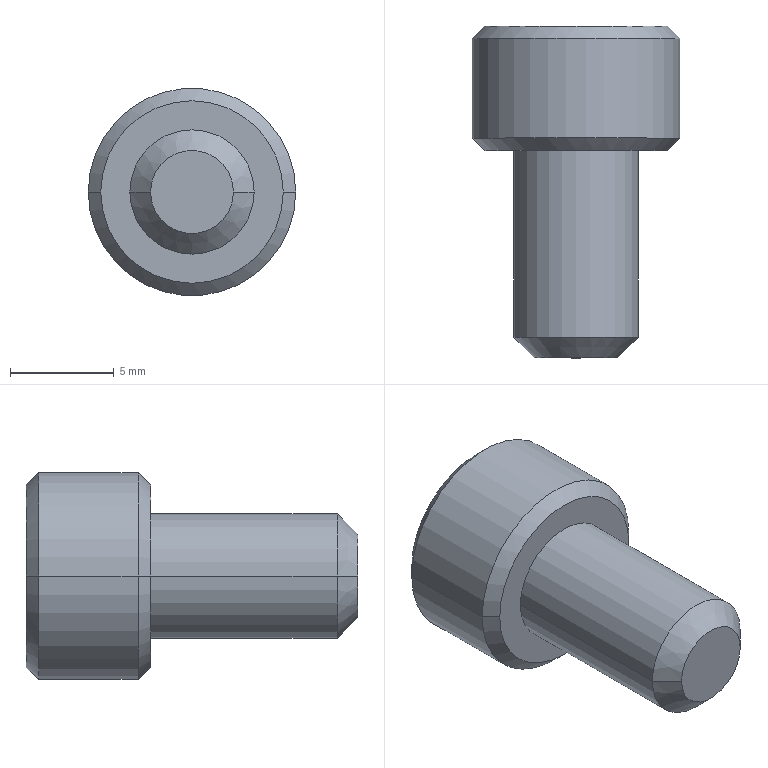Part | STEP file | BB62-M6-10L-3 | 1 solid | 27 faces | box 10 x 16 x 10 mm | volume 656.85 mm3 | plane 15 | cone 8 | cylinder 4 | commonest cylinder face diameters 6 x2 10 x2
STEP:
#1=CARTESIAN_POINT('',(0.,1.349,0.));
#2=VERTEX_POINT('',#1);
#3=CARTESIAN_POINT('',(2.86,3.,0.));
#4=VERTEX_POINT('',#3);
#5=CARTESIAN_POINT('',(0.,1.349,0.));
#6=DIRECTION('',(0.866,0.5,0.));
#7=VECTOR('',#6,1000.);
#8=LINE('',#5,#7);
#9=EDGE_CURVE('',#2,#4,#8,.T.);
#10=ORIENTED_EDGE('',*,*,#9,.F.);
#11=CARTESIAN_POINT('',(-2.86,3.,0.));
#12=VERTEX_POINT('',#11);
#13=CARTESIAN_POINT('',(0.,1.349,0.));
#14=DIRECTION('',(-0.866,0.5,0.));
#15=VECTOR('',#14,1000.);
#16=LINE('',#13,#15);
#17=EDGE_CURVE('',#2,#12,#16,.T.);
#18=ORIENTED_EDGE('',*,*,#17,.T.);
#19=CARTESIAN_POINT('',(-2.477,3.,1.43));
#20=VERTEX_POINT('',#19);
#21=CARTESIAN_POINT('',(0.,3.,0.));
#22=DIRECTION('',(0.,-1.,0.));
#23=DIRECTION('',(-1.,0.,0.));
#24=AXIS2_PLACEMENT_3D('',#21,#22,#23);
#25=CIRCLE('',#24,2.86);
#26=EDGE_CURVE('',#20,#12,#25,.T.);
#27=ORIENTED_EDGE('',*,*,#26,.F.);
#28=CARTESIAN_POINT('',(0.,3.,2.86));
#29=VERTEX_POINT('',#28);
#30=CARTESIAN_POINT('',(0.,3.,0.));
#31=DIRECTION('',(0.,-1.,0.));
#32=DIRECTION('',(-1.,0.,0.));
#33=AXIS2_PLACEMENT_3D('',#30,#31,#32);
#34=CIRCLE('',#33,2.86);
#35=EDGE_CURVE('',#29,#20,#34,.T.);
#36=ORIENTED_EDGE('',*,*,#35,.F.);
#37=CARTESIAN_POINT('',(2.477,3.,1.43));
#38=VERTEX_POINT('',#37);
#39=CARTESIAN_POINT('',(0.,3.,0.));
#40=DIRECTION('',(0.,-1.,0.));
#41=DIRECTION('',(-1.,0.,0.));
#42=AXIS2_PLACEMENT_3D('',#39,#40,#41);
#43=CIRCLE('',#42,2.86);
#44=EDGE_CURVE('',#38,#29,#43,.T.);
#45=ORIENTED_EDGE('',*,*,#44,.F.);
#46=CARTESIAN_POINT('',(0.,3.,0.));
#47=DIRECTION('',(0.,-1.,0.));
#48=DIRECTION('',(-1.,0.,0.));
#49=AXIS2_PLACEMENT_3D('',#46,#47,#48);
#50=CIRCLE('',#49,2.86);
#51=EDGE_CURVE('',#4,#38,#50,.T.);
#52=ORIENTED_EDGE('',*,*,#51,.F.);
#53=EDGE_LOOP('',(#10,#18,#27,#36,#45,#52));
#54=FACE_OUTER_BOUND('',#53,.T.);
#55=CARTESIAN_POINT('',(0.,1001.349,0.));
#56=DIRECTION('',(0.,1.,0.));
#57=DIRECTION('',(1.,0.,0.));
#58=AXIS2_PLACEMENT_3D('',#55,#56,#57);
#59=CONICAL_SURFACE('',#58,1732.051,1.047);
#60=ADVANCED_FACE('',(#54),#59,.F.);
#61=CARTESIAN_POINT('',(2.,-10.,0.));
#62=VERTEX_POINT('',#61);
#63=CARTESIAN_POINT('',(-2.,-10.,0.));
#64=VERTEX_POINT('',#63);
#65=CARTESIAN_POINT('',(0.,-10.,0.));
#66=DIRECTION('',(0.,1.,0.));
#67=DIRECTION('',(1.,0.,0.));
#68=AXIS2_PLACEMENT_3D('',#65,#66,#67);
#69=CIRCLE('',#68,2.);
#70=EDGE_CURVE('',#62,#64,#69,.T.);
#71=ORIENTED_EDGE('',*,*,#70,.T.);
#72=CARTESIAN_POINT('',(-3.,-9.,0.));
#73=VERTEX_POINT('',#72);
#74=CARTESIAN_POINT('',(-2.,-10.,0.));
#75=DIRECTION('',(-0.7071,0.7071,0.));
#76=VECTOR('',#75,1000.);
#77=LINE('',#74,#76);
#78=EDGE_CURVE('',#64,#73,#77,.T.);
#79=ORIENTED_EDGE('',*,*,#78,.T.);
#80=CARTESIAN_POINT('',(3.,-9.,0.));
#81=VERTEX_POINT('',#80);
#82=CARTESIAN_POINT('',(0.,-9.,0.));
#83=DIRECTION('',(0.,-1.,0.));
#84=DIRECTION('',(-1.,0.,0.));
#85=AXIS2_PLACEMENT_3D('',#82,#83,#84);
#86=CIRCLE('',#85,3.);
#87=EDGE_CURVE('',#73,#81,#86,.T.);
#88=ORIENTED_EDGE('',*,*,#87,.T.);
#89=CARTESIAN_POINT('',(2.,-10.,0.));
#90=DIRECTION('',(0.7071,0.7071,0.));
#91=VECTOR('',#90,1000.);
#92=LINE('',#89,#91);
#93=EDGE_CURVE('',#62,#81,#92,.T.);
#94=ORIENTED_EDGE('',*,*,#93,.F.);
#95=EDGE_LOOP('',(#71,#79,#88,#94));
#96=FACE_OUTER_BOUND('',#95,.T.);
#97=CARTESIAN_POINT('',(0.,-10.,0.));
#98=DIRECTION('',(0.,1.,0.));
#99=DIRECTION('',(1.,0.,0.));
#100=AXIS2_PLACEMENT_3D('',#97,#98,#99);
#101=CONICAL_SURFACE('',#100,2.,0.7854);
#102=ADVANCED_FACE('',(#96),#101,.T.);
#103=ORIENTED_EDGE('',*,*,#87,.F.);
#104=CARTESIAN_POINT('',(-3.,0.,0.));
#105=VERTEX_POINT('',#104);
#106=CARTESIAN_POINT('',(-3.,-9.,0.));
#107=DIRECTION('',(0.,1.,0.));
#108=VECTOR('',#107,1000.);
#109=LINE('',#106,#108);
#110=EDGE_CURVE('',#73,#105,#109,.T.);
#111=ORIENTED_EDGE('',*,*,#110,.T.);
#112=CARTESIAN_POINT('',(3.,0.,0.));
#113=VERTEX_POINT('',#112);
#114=CARTESIAN_POINT('',(0.,0.,0.));
#115=DIRECTION('',(0.,-1.,0.));
#116=DIRECTION('',(-1.,0.,0.));
#117=AXIS2_PLACEMENT_3D('',#114,#115,#116);
#118=CIRCLE('',#117,3.);
#119=EDGE_CURVE('',#105,#113,#118,.T.);
#120=ORIENTED_EDGE('',*,*,#119,.T.);
#121=CARTESIAN_POINT('',(3.,-9.,0.));
#122=DIRECTION('',(0.,1.,0.));
#123=VECTOR('',#122,1000.);
#124=LINE('',#121,#123);
#125=EDGE_CURVE('',#81,#113,#124,.T.);
#126=ORIENTED_EDGE('',*,*,#125,.F.);
#127=EDGE_LOOP('',(#103,#111,#120,#126));
#128=FACE_OUTER_BOUND('',#127,.T.);
#129=CARTESIAN_POINT('',(0.,-9.,0.));
#130=DIRECTION('',(0.,1.,0.));
#131=DIRECTION('',(1.,0.,0.));
#132=AXIS2_PLACEMENT_3D('',#129,#130,#131);
#133=CYLINDRICAL_SURFACE('',#132,3.);
#134=ADVANCED_FACE('',(#128),#133,.T.);
#135=CARTESIAN_POINT('',(-4.4,6.,0.));
#136=VERTEX_POINT('',#135);
#137=CARTESIAN_POINT('',(4.4,6.,0.));
#138=VERTEX_POINT('',#137);
#139=CARTESIAN_POINT('',(0.,6.,0.));
#140=DIRECTION('',(0.,-1.,0.));
#141=DIRECTION('',(-1.,0.,0.));
#142=AXIS2_PLACEMENT_3D('',#139,#140,#141);
#143=CIRCLE('',#142,4.4);
#144=EDGE_CURVE('',#136,#138,#143,.T.);
#145=ORIENTED_EDGE('',*,*,#144,.T.);
#146=CARTESIAN_POINT('',(5.,5.4,0.));
#147=VERTEX_POINT('',#146);
#148=CARTESIAN_POINT('',(5.,5.4,0.));
#149=DIRECTION('',(0.7071,-0.7071,0.));
#150=VECTOR('',#149,1000.);
#151=LINE('',#148,#150);
#152=EDGE_CURVE('',#138,#147,#151,.T.);
#153=ORIENTED_EDGE('',*,*,#152,.T.);
#154=CARTESIAN_POINT('',(-5.,5.4,0.));
#155=VERTEX_POINT('',#154);
#156=CARTESIAN_POINT('',(0.,5.4,0.));
#157=DIRECTION('',(0.,-1.,0.));
#158=DIRECTION('',(-1.,0.,0.));
#159=AXIS2_PLACEMENT_3D('',#156,#157,#158);
#160=CIRCLE('',#159,5.);
#161=EDGE_CURVE('',#155,#147,#160,.T.);
#162=ORIENTED_EDGE('',*,*,#161,.F.);
#163=CARTESIAN_POINT('',(-5.,5.4,0.));
#164=DIRECTION('',(-0.7071,-0.7071,0.));
#165=VECTOR('',#164,1000.);
#166=LINE('',#163,#165);
#167=EDGE_CURVE('',#136,#155,#166,.T.);
#168=ORIENTED_EDGE('',*,*,#167,.F.);
#169=EDGE_LOOP('',(#145,#153,#162,#168));
#170=FACE_OUTER_BOUND('',#169,.T.);
#171=CARTESIAN_POINT('',(0.,5.4,0.));
#172=DIRECTION('',(0.,-1.,0.));
#173=DIRECTION('',(-1.,0.,0.));
#174=AXIS2_PLACEMENT_3D('',#171,#172,#173);
#175=CONICAL_SURFACE('',#174,5.,0.7854);
#176=ADVANCED_FACE('',(#170),#175,.T.);
#177=ORIENTED_EDGE('',*,*,#161,.T.);
#178=CARTESIAN_POINT('',(5.,0.6,0.));
#179=VERTEX_POINT('',#178);
#180=CARTESIAN_POINT('',(5.,1.62,0.));
#181=DIRECTION('',(0.,-1.,0.));
#182=VECTOR('',#181,1000.);
#183=LINE('',#180,#182);
#184=EDGE_CURVE('',#147,#179,#183,.T.);
#185=ORIENTED_EDGE('',*,*,#184,.T.);
#186=CARTESIAN_POINT('',(-5.,0.6,0.));
#187=VERTEX_POINT('',#186);
#188=CARTESIAN_POINT('',(0.,0.6,0.));
#189=DIRECTION('',(0.,-1.,0.));
#190=DIRECTION('',(-1.,0.,0.));
#191=AXIS2_PLACEMENT_3D('',#188,#189,#190);
#192=CIRCLE('',#191,5.);
#193=EDGE_CURVE('',#187,#179,#192,.T.);
#194=ORIENTED_EDGE('',*,*,#193,.F.);
#195=CARTESIAN_POINT('',(-5.,1.62,0.));
#196=DIRECTION('',(0.,-1.,0.));
#197=VECTOR('',#196,1000.);
#198=LINE('',#195,#197);
#199=EDGE_CURVE('',#155,#187,#198,.T.);
#200=ORIENTED_EDGE('',*,*,#199,.F.);
#201=EDGE_LOOP('',(#177,#185,#194,#200));
#202=FACE_OUTER_BOUND('',#201,.T.);
#203=CARTESIAN_POINT('',(0.,1.62,0.));
#204=DIRECTION('',(0.,-1.,0.));
#205=DIRECTION('',(-1.,0.,0.));
#206=AXIS2_PLACEMENT_3D('',#203,#204,#205);
#207=CYLINDRICAL_SURFACE('',#206,5.);
#208=ADVANCED_FACE('',(#202),#207,.T.);
#209=CARTESIAN_POINT('',(-4.4,0.,0.));
#210=VERTEX_POINT('',#209);
#211=CARTESIAN_POINT('',(4.4,0.,0.));
#212=VERTEX_POINT('',#211);
#213=CARTESIAN_POINT('',(0.,0.,0.));
#214=DIRECTION('',(0.,-1.,0.));
#215=DIRECTION('',(-1.,0.,0.));
#216=AXIS2_PLACEMENT_3D('',#213,#214,#215);
#217=CIRCLE('',#216,4.4);
#218=EDGE_CURVE('',#210,#212,#217,.T.);
#219=ORIENTED_EDGE('',*,*,#218,.F.);
#220=CARTESIAN_POINT('',(-4.4,0.,0.));
#221=DIRECTION('',(-0.7071,0.7071,0.));
#222=VECTOR('',#221,1000.);
#223=LINE('',#220,#222);
#224=EDGE_CURVE('',#210,#187,#223,.T.);
#225=ORIENTED_EDGE('',*,*,#224,.T.);
#226=ORIENTED_EDGE('',*,*,#193,.T.);
#227=CARTESIAN_POINT('',(4.4,0.,0.));
#228=DIRECTION('',(0.7071,0.7071,0.));
#229=VECTOR('',#228,1000.);
#230=LINE('',#227,#229);
#231=EDGE_CURVE('',#212,#179,#230,.T.);
#232=ORIENTED_EDGE('',*,*,#231,.F.);
#233=EDGE_LOOP('',(#219,#225,#226,#232));
#234=FACE_OUTER_BOUND('',#233,.T.);
#235=CARTESIAN_POINT('',(0.,0.,0.));
#236=DIRECTION('',(0.,1.,0.));
#237=DIRECTION('',(1.,0.,0.));
#238=AXIS2_PLACEMENT_3D('',#235,#236,#237);
#239=CONICAL_SURFACE('',#238,4.4,0.7854);
#240=ADVANCED_FACE('',(#234),#239,.T.);
#241=ORIENTED_EDGE('',*,*,#144,.F.);
#242=CARTESIAN_POINT('',(0.,6.,0.));
#243=DIRECTION('',(0.,-1.,0.));
#244=DIRECTION('',(-1.,0.,0.));
#245=AXIS2_PLACEMENT_3D('',#242,#243,#244);
#246=CIRCLE('',#245,4.4);
#247=EDGE_CURVE('',#138,#136,#246,.T.);
#248=ORIENTED_EDGE('',*,*,#247,.F.);
#249=EDGE_LOOP('',(#241,#248));
#250=FACE_OUTER_BOUND('',#249,.T.);
#251=CARTESIAN_POINT('',(0.,6.,-2.86));
#252=VERTEX_POINT('',#251);
#253=CARTESIAN_POINT('',(-2.477,6.,-1.43));
#254=VERTEX_POINT('',#253);
#255=CARTESIAN_POINT('',(0.,6.,-2.86));
#256=DIRECTION('',(-0.866,0.,0.5));
#257=VECTOR('',#256,1000.);
#258=LINE('',#255,#257);
#259=EDGE_CURVE('',#252,#254,#258,.T.);
#260=ORIENTED_EDGE('',*,*,#259,.F.);
#261=CARTESIAN_POINT('',(2.477,6.,-1.43));
#262=VERTEX_POINT('',#261);
#263=CARTESIAN_POINT('',(2.477,6.,-1.43));
#264=DIRECTION('',(-0.866,0.,-0.5));
#265=VECTOR('',#264,1000.);
#266=LINE('',#263,#265);
#267=EDGE_CURVE('',#262,#252,#266,.T.);
#268=ORIENTED_EDGE('',*,*,#267,.F.);
#269=CARTESIAN_POINT('',(2.477,6.,1.43));
#270=VERTEX_POINT('',#269);
#271=CARTESIAN_POINT('',(2.477,6.,1.43));
#272=DIRECTION('',(0.,0.,-1.));
#273=VECTOR('',#272,1000.);
#274=LINE('',#271,#273);
#275=EDGE_CURVE('',#270,#262,#274,.T.);
#276=ORIENTED_EDGE('',*,*,#275,.F.);
#277=CARTESIAN_POINT('',(0.,6.,2.86));
#278=VERTEX_POINT('',#277);
#279=CARTESIAN_POINT('',(0.,6.,2.86));
#280=DIRECTION('',(0.866,0.,-0.5));
#281=VECTOR('',#280,1000.);
#282=LINE('',#279,#281);
#283=EDGE_CURVE('',#278,#270,#282,.T.);
#284=ORIENTED_EDGE('',*,*,#283,.F.);
#285=CARTESIAN_POINT('',(-2.477,6.,1.43));
#286=VERTEX_POINT('',#285);
#287=CARTESIAN_POINT('',(-2.477,6.,1.43));
#288=DIRECTION('',(0.866,0.,0.5));
#289=VECTOR('',#288,1000.);
#290=LINE('',#287,#289);
#291=EDGE_CURVE('',#286,#278,#290,.T.);
#292=ORIENTED_EDGE('',*,*,#291,.F.);
#293=CARTESIAN_POINT('',(-2.477,6.,-1.43));
#294=DIRECTION('',(0.,0.,1.));
#295=VECTOR('',#294,1000.);
#296=LINE('',#293,#295);
#297=EDGE_CURVE('',#254,#286,#296,.T.);
#298=ORIENTED_EDGE('',*,*,#297,.F.);
#299=EDGE_LOOP('',(#260,#268,#276,#284,#292,#298));
#300=FACE_BOUND('',#299,.T.);
#301=CARTESIAN_POINT('',(4.4,6.,0.));
#302=DIRECTION('',(0.,1.,0.));
#303=DIRECTION('',(1.,0.,0.));
#304=AXIS2_PLACEMENT_3D('',#301,#302,#303);
#305=PLANE('',#304);
#306=ADVANCED_FACE('',(#250,#300),#305,.T.);
#307=CARTESIAN_POINT('',(0.,0.,0.));
#308=DIRECTION('',(0.,-1.,0.));
#309=DIRECTION('',(-1.,0.,0.));
#310=AXIS2_PLACEMENT_3D('',#307,#308,#309);
#311=CIRCLE('',#310,3.);
#312=EDGE_CURVE('',#113,#105,#311,.T.);
#313=ORIENTED_EDGE('',*,*,#312,.F.);
#314=ORIENTED_EDGE('',*,*,#119,.F.);
#315=EDGE_LOOP('',(#313,#314));
#316=FACE_BOUND('',#315,.T.);
#317=CARTESIAN_POINT('',(0.,0.,0.));
#318=DIRECTION('',(0.,-1.,0.));
#319=DIRECTION('',(-1.,0.,0.));
#320=AXIS2_PLACEMENT_3D('',#317,#318,#319);
#321=CIRCLE('',#320,4.4);
#322=EDGE_CURVE('',#212,#210,#321,.T.);
#323=ORIENTED_EDGE('',*,*,#322,.T.);
#324=ORIENTED_EDGE('',*,*,#218,.T.);
#325=EDGE_LOOP('',(#323,#324));
#326=FACE_OUTER_BOUND('',#325,.T.);
#327=CARTESIAN_POINT('',(0.,0.,0.));
#328=DIRECTION('',(0.,-1.,0.));
#329=DIRECTION('',(-1.,0.,0.));
#330=AXIS2_PLACEMENT_3D('',#327,#328,#329);
#331=PLANE('',#330);
#332=ADVANCED_FACE('',(#316,#326),#331,.T.);
#333=ORIENTED_EDGE('',*,*,#224,.F.);
#334=ORIENTED_EDGE('',*,*,#322,.F.);
#335=ORIENTED_EDGE('',*,*,#231,.T.);
#336=CARTESIAN_POINT('',(0.,0.6,0.));
#337=DIRECTION('',(0.,-1.,0.));
#338=DIRECTION('',(-1.,0.,0.));
#339=AXIS2_PLACEMENT_3D('',#336,#337,#338);
#340=CIRCLE('',#339,5.);
#341=EDGE_CURVE('',#179,#187,#340,.T.);
#342=ORIENTED_EDGE('',*,*,#341,.T.);
#343=EDGE_LOOP('',(#333,#334,#335,#342));
#344=FACE_OUTER_BOUND('',#343,.T.);
#345=CARTESIAN_POINT('',(0.,0.,0.));
#346=DIRECTION('',(0.,1.,0.));
#347=DIRECTION('',(1.,0.,0.));
#348=AXIS2_PLACEMENT_3D('',#345,#346,#347);
#349=CONICAL_SURFACE('',#348,4.4,0.7854);
#350=ADVANCED_FACE('',(#344),#349,.T.);
#351=ORIENTED_EDGE('',*,*,#184,.F.);
#352=CARTESIAN_POINT('',(0.,5.4,0.));
#353=DIRECTION('',(0.,-1.,0.));
#354=DIRECTION('',(-1.,0.,0.));
#355=AXIS2_PLACEMENT_3D('',#352,#353,#354);
#356=CIRCLE('',#355,5.);
#357=EDGE_CURVE('',#147,#155,#356,.T.);
#358=ORIENTED_EDGE('',*,*,#357,.T.);
#359=ORIENTED_EDGE('',*,*,#199,.T.);
#360=ORIENTED_EDGE('',*,*,#341,.F.);
#361=EDGE_LOOP('',(#351,#358,#359,#360));
#362=FACE_OUTER_BOUND('',#361,.T.);
#363=CARTESIAN_POINT('',(0.,1.62,0.));
#364=DIRECTION('',(0.,-1.,0.));
#365=DIRECTION('',(-1.,0.,0.));
#366=AXIS2_PLACEMENT_3D('',#363,#364,#365);
#367=CYLINDRICAL_SURFACE('',#366,5.);
#368=ADVANCED_FACE('',(#362),#367,.T.);
#369=ORIENTED_EDGE('',*,*,#152,.F.);
#370=ORIENTED_EDGE('',*,*,#247,.T.);
#371=ORIENTED_EDGE('',*,*,#167,.T.);
#372=ORIENTED_EDGE('',*,*,#357,.F.);
#373=EDGE_LOOP('',(#369,#370,#371,#372));
#374=FACE_OUTER_BOUND('',#373,.T.);
#375=CARTESIAN_POINT('',(0.,5.4,0.));
#376=DIRECTION('',(0.,-1.,0.));
#377=DIRECTION('',(-1.,0.,0.));
#378=AXIS2_PLACEMENT_3D('',#375,#376,#377);
#379=CONICAL_SURFACE('',#378,5.,0.7854);
#380=ADVANCED_FACE('',(#374),#379,.T.);
#381=ORIENTED_EDGE('',*,*,#110,.F.);
#382=CARTESIAN_POINT('',(0.,-9.,0.));
#383=DIRECTION('',(0.,-1.,0.));
#384=DIRECTION('',(-1.,0.,0.));
#385=AXIS2_PLACEMENT_3D('',#382,#383,#384);
#386=CIRCLE('',#385,3.);
#387=EDGE_CURVE('',#81,#73,#386,.T.);
#388=ORIENTED_EDGE('',*,*,#387,.F.);
#389=ORIENTED_EDGE('',*,*,#125,.T.);
#390=ORIENTED_EDGE('',*,*,#312,.T.);
#391=EDGE_LOOP('',(#381,#388,#389,#390));
#392=FACE_OUTER_BOUND('',#391,.T.);
#393=CARTESIAN_POINT('',(0.,-9.,0.));
#394=DIRECTION('',(0.,1.,0.));
#395=DIRECTION('',(1.,0.,0.));
#396=AXIS2_PLACEMENT_3D('',#393,#394,#395);
#397=CYLINDRICAL_SURFACE('',#396,3.);
#398=ADVANCED_FACE('',(#392),#397,.T.);
#399=ORIENTED_EDGE('',*,*,#70,.F.);
#400=CARTESIAN_POINT('',(0.,-10.,0.));
#401=DIRECTION('',(0.,1.,0.));
#402=DIRECTION('',(1.,0.,0.));
#403=AXIS2_PLACEMENT_3D('',#400,#401,#402);
#404=CIRCLE('',#403,2.);
#405=EDGE_CURVE('',#64,#62,#404,.T.);
#406=ORIENTED_EDGE('',*,*,#405,.F.);
#407=EDGE_LOOP('',(#399,#406));
#408=FACE_OUTER_BOUND('',#407,.T.);
#409=CARTESIAN_POINT('',(0.,-10.,0.));
#410=DIRECTION('',(0.,-1.,0.));
#411=DIRECTION('',(-1.,0.,0.));
#412=AXIS2_PLACEMENT_3D('',#409,#410,#411);
#413=PLANE('',#412);
#414=ADVANCED_FACE('',(#408),#413,.T.);
#415=ORIENTED_EDGE('',*,*,#78,.F.);
#416=ORIENTED_EDGE('',*,*,#405,.T.);
#417=ORIENTED_EDGE('',*,*,#93,.T.);
#418=ORIENTED_EDGE('',*,*,#387,.T.);
#419=EDGE_LOOP('',(#415,#416,#417,#418));
#420=FACE_OUTER_BOUND('',#419,.T.);
#421=CARTESIAN_POINT('',(0.,-10.,0.));
#422=DIRECTION('',(0.,1.,0.));
#423=DIRECTION('',(1.,0.,0.));
#424=AXIS2_PLACEMENT_3D('',#421,#422,#423);
#425=CONICAL_SURFACE('',#424,2.,0.7854);
#426=ADVANCED_FACE('',(#420),#425,.T.);
#427=CARTESIAN_POINT('',(2.477,3.,-1.43));
#428=VERTEX_POINT('',#427);
#429=CARTESIAN_POINT('',(0.,3.,-2.86));
#430=VERTEX_POINT('',#429);
#431=CARTESIAN_POINT('',(2.477,3.,-1.43));
#432=DIRECTION('',(-0.866,0.,-0.5));
#433=VECTOR('',#432,1000.);
#434=LINE('',#431,#433);
#435=EDGE_CURVE('',#428,#430,#434,.T.);
#436=ORIENTED_EDGE('',*,*,#435,.F.);
#437=CARTESIAN_POINT('',(2.477,6.,-1.43));
#438=DIRECTION('',(0.,-1.,0.));
#439=VECTOR('',#438,1000.);
#440=LINE('',#437,#439);
#441=EDGE_CURVE('',#262,#428,#440,.T.);
#442=ORIENTED_EDGE('',*,*,#441,.F.);
#443=ORIENTED_EDGE('',*,*,#267,.T.);
#444=CARTESIAN_POINT('',(0.,6.,-2.86));
#445=DIRECTION('',(0.,-1.,0.));
#446=VECTOR('',#445,1000.);
#447=LINE('',#444,#446);
#448=EDGE_CURVE('',#252,#430,#447,.T.);
#449=ORIENTED_EDGE('',*,*,#448,.T.);
#450=EDGE_LOOP('',(#436,#442,#443,#449));
#451=FACE_OUTER_BOUND('',#450,.T.);
#452=CARTESIAN_POINT('',(2.477,6.,-1.43));
#453=DIRECTION('',(-0.5,0.,0.866));
#454=DIRECTION('',(0.866,0.,0.5));
#455=AXIS2_PLACEMENT_3D('',#452,#453,#454);
#456=PLANE('',#455);
#457=ADVANCED_FACE('',(#451),#456,.T.);
#458=CARTESIAN_POINT('',(-2.477,3.,-1.43));
#459=VERTEX_POINT('',#458);
#460=CARTESIAN_POINT('',(0.,3.,-2.86));
#461=DIRECTION('',(-0.866,0.,0.5));
#462=VECTOR('',#461,1000.);
#463=LINE('',#460,#462);
#464=EDGE_CURVE('',#430,#459,#463,.T.);
#465=ORIENTED_EDGE('',*,*,#464,.F.);
#466=ORIENTED_EDGE('',*,*,#448,.F.);
#467=ORIENTED_EDGE('',*,*,#259,.T.);
#468=CARTESIAN_POINT('',(-2.477,6.,-1.43));
#469=DIRECTION('',(0.,-1.,0.));
#470=VECTOR('',#469,1000.);
#471=LINE('',#468,#470);
#472=EDGE_CURVE('',#254,#459,#471,.T.);
#473=ORIENTED_EDGE('',*,*,#472,.T.);
#474=EDGE_LOOP('',(#465,#466,#467,#473));
#475=FACE_OUTER_BOUND('',#474,.T.);
#476=CARTESIAN_POINT('',(0.,6.,-2.86));
#477=DIRECTION('',(0.5,0.,0.866));
#478=DIRECTION('',(0.866,0.,-0.5));
#479=AXIS2_PLACEMENT_3D('',#476,#477,#478);
#480=PLANE('',#479);
#481=ADVANCED_FACE('',(#475),#480,.T.);
#482=CARTESIAN_POINT('',(-2.477,3.,-1.43));
#483=DIRECTION('',(0.,0.,1.));
#484=VECTOR('',#483,1000.);
#485=LINE('',#482,#484);
#486=EDGE_CURVE('',#459,#20,#485,.T.);
#487=ORIENTED_EDGE('',*,*,#486,.F.);
#488=ORIENTED_EDGE('',*,*,#472,.F.);
#489=ORIENTED_EDGE('',*,*,#297,.T.);
#490=CARTESIAN_POINT('',(-2.477,6.,1.43));
#491=DIRECTION('',(0.,-1.,0.));
#492=VECTOR('',#491,1000.);
#493=LINE('',#490,#492);
#494=EDGE_CURVE('',#286,#20,#493,.T.);
#495=ORIENTED_EDGE('',*,*,#494,.T.);
#496=EDGE_LOOP('',(#487,#488,#489,#495));
#497=FACE_OUTER_BOUND('',#496,.T.);
#498=CARTESIAN_POINT('',(-2.477,6.,-1.43));
#499=DIRECTION('',(1.,0.,0.));
#500=DIRECTION('',(0.,0.,-1.));
#501=AXIS2_PLACEMENT_3D('',#498,#499,#500);
#502=PLANE('',#501);
#503=ADVANCED_FACE('',(#497),#502,.T.);
#504=CARTESIAN_POINT('',(-2.477,3.,1.43));
#505=DIRECTION('',(0.866,0.,0.5));
#506=VECTOR('',#505,1000.);
#507=LINE('',#504,#506);
#508=EDGE_CURVE('',#20,#29,#507,.T.);
#509=ORIENTED_EDGE('',*,*,#508,.F.);
#510=ORIENTED_EDGE('',*,*,#494,.F.);
#511=ORIENTED_EDGE('',*,*,#291,.T.);
#512=CARTESIAN_POINT('',(0.,6.,2.86));
#513=DIRECTION('',(0.,-1.,0.));
#514=VECTOR('',#513,1000.);
#515=LINE('',#512,#514);
#516=EDGE_CURVE('',#278,#29,#515,.T.);
#517=ORIENTED_EDGE('',*,*,#516,.T.);
#518=EDGE_LOOP('',(#509,#510,#511,#517));
#519=FACE_OUTER_BOUND('',#518,.T.);
#520=CARTESIAN_POINT('',(-2.477,6.,1.43));
#521=DIRECTION('',(0.5,0.,-0.866));
#522=DIRECTION('',(-0.866,0.,-0.5));
#523=AXIS2_PLACEMENT_3D('',#520,#521,#522);
#524=PLANE('',#523);
#525=ADVANCED_FACE('',(#519),#524,.T.);
#526=CARTESIAN_POINT('',(0.,3.,2.86));
#527=DIRECTION('',(0.866,0.,-0.5));
#528=VECTOR('',#527,1000.);
#529=LINE('',#526,#528);
#530=EDGE_CURVE('',#29,#38,#529,.T.);
#531=ORIENTED_EDGE('',*,*,#530,.F.);
#532=ORIENTED_EDGE('',*,*,#516,.F.);
#533=ORIENTED_EDGE('',*,*,#283,.T.);
#534=CARTESIAN_POINT('',(2.477,6.,1.43));
#535=DIRECTION('',(0.,-1.,0.));
#536=VECTOR('',#535,1000.);
#537=LINE('',#534,#536);
#538=EDGE_CURVE('',#270,#38,#537,.T.);
#539=ORIENTED_EDGE('',*,*,#538,.T.);
#540=EDGE_LOOP('',(#531,#532,#533,#539));
#541=FACE_OUTER_BOUND('',#540,.T.);
#542=CARTESIAN_POINT('',(0.,6.,2.86));
#543=DIRECTION('',(-0.5,0.,-0.866));
#544=DIRECTION('',(-0.866,0.,0.5));
#545=AXIS2_PLACEMENT_3D('',#542,#543,#544);
#546=PLANE('',#545);
#547=ADVANCED_FACE('',(#541),#546,.T.);
#548=CARTESIAN_POINT('',(2.477,3.,1.43));
#549=DIRECTION('',(0.,0.,-1.));
#550=VECTOR('',#549,1000.);
#551=LINE('',#548,#550);
#552=EDGE_CURVE('',#38,#428,#551,.T.);
#553=ORIENTED_EDGE('',*,*,#552,.F.);
#554=ORIENTED_EDGE('',*,*,#538,.F.);
#555=ORIENTED_EDGE('',*,*,#275,.T.);
#556=ORIENTED_EDGE('',*,*,#441,.T.);
#557=EDGE_LOOP('',(#553,#554,#555,#556));
#558=FACE_OUTER_BOUND('',#557,.T.);
#559=CARTESIAN_POINT('',(2.477,6.,1.43));
#560=DIRECTION('',(-1.,0.,0.));
#561=DIRECTION('',(0.,0.,1.));
#562=AXIS2_PLACEMENT_3D('',#559,#560,#561);
#563=PLANE('',#562);
#564=ADVANCED_FACE('',(#558),#563,.T.);
#565=ORIENTED_EDGE('',*,*,#435,.T.);
#566=CARTESIAN_POINT('',(0.,3.,0.));
#567=DIRECTION('',(0.,-1.,0.));
#568=DIRECTION('',(-1.,0.,0.));
#569=AXIS2_PLACEMENT_3D('',#566,#567,#568);
#570=CIRCLE('',#569,2.86);
#571=EDGE_CURVE('',#430,#428,#570,.T.);
#572=ORIENTED_EDGE('',*,*,#571,.T.);
#573=EDGE_LOOP('',(#565,#572));
#574=FACE_OUTER_BOUND('',#573,.T.);
#575=CARTESIAN_POINT('',(0.,3.,0.));
#576=DIRECTION('',(0.,1.,0.));
#577=DIRECTION('',(1.,0.,0.));
#578=AXIS2_PLACEMENT_3D('',#575,#576,#577);
#579=PLANE('',#578);
#580=ADVANCED_FACE('',(#574),#579,.F.);
#581=ORIENTED_EDGE('',*,*,#552,.T.);
#582=CARTESIAN_POINT('',(0.,3.,0.));
#583=DIRECTION('',(0.,-1.,0.));
#584=DIRECTION('',(-1.,0.,0.));
#585=AXIS2_PLACEMENT_3D('',#582,#583,#584);
#586=CIRCLE('',#585,2.86);
#587=EDGE_CURVE('',#428,#4,#586,.T.);
#588=ORIENTED_EDGE('',*,*,#587,.T.);
#589=ORIENTED_EDGE('',*,*,#51,.T.);
#590=EDGE_LOOP('',(#581,#588,#589));
#591=FACE_OUTER_BOUND('',#590,.T.);
#592=CARTESIAN_POINT('',(0.,3.,0.));
#593=DIRECTION('',(0.,1.,0.));
#594=DIRECTION('',(1.,0.,0.));
#595=AXIS2_PLACEMENT_3D('',#592,#593,#594);
#596=PLANE('',#595);
#597=ADVANCED_FACE('',(#591),#596,.F.);
#598=ORIENTED_EDGE('',*,*,#530,.T.);
#599=ORIENTED_EDGE('',*,*,#44,.T.);
#600=EDGE_LOOP('',(#598,#599));
#601=FACE_OUTER_BOUND('',#600,.T.);
#602=CARTESIAN_POINT('',(0.,3.,0.));
#603=DIRECTION('',(0.,1.,0.));
#604=DIRECTION('',(1.,0.,0.));
#605=AXIS2_PLACEMENT_3D('',#602,#603,#604);
#606=PLANE('',#605);
#607=ADVANCED_FACE('',(#601),#606,.F.);
#608=ORIENTED_EDGE('',*,*,#508,.T.);
#609=ORIENTED_EDGE('',*,*,#35,.T.);
#610=EDGE_LOOP('',(#608,#609));
#611=FACE_OUTER_BOUND('',#610,.T.);
#612=CARTESIAN_POINT('',(0.,3.,0.));
#613=DIRECTION('',(0.,1.,0.));
#614=DIRECTION('',(1.,0.,0.));
#615=AXIS2_PLACEMENT_3D('',#612,#613,#614);
#616=PLANE('',#615);
#617=ADVANCED_FACE('',(#611),#616,.F.);
#618=ORIENTED_EDGE('',*,*,#486,.T.);
#619=ORIENTED_EDGE('',*,*,#26,.T.);
#620=CARTESIAN_POINT('',(0.,3.,0.));
#621=DIRECTION('',(0.,-1.,0.));
#622=DIRECTION('',(-1.,0.,0.));
#623=AXIS2_PLACEMENT_3D('',#620,#621,#622);
#624=CIRCLE('',#623,2.86);
#625=EDGE_CURVE('',#12,#459,#624,.T.);
#626=ORIENTED_EDGE('',*,*,#625,.T.);
#627=EDGE_LOOP('',(#618,#619,#626));
#628=FACE_OUTER_BOUND('',#627,.T.);
#629=CARTESIAN_POINT('',(0.,3.,0.));
#630=DIRECTION('',(0.,1.,0.));
#631=DIRECTION('',(1.,0.,0.));
#632=AXIS2_PLACEMENT_3D('',#629,#630,#631);
#633=PLANE('',#632);
#634=ADVANCED_FACE('',(#628),#633,.F.);
#635=ORIENTED_EDGE('',*,*,#464,.T.);
#636=CARTESIAN_POINT('',(0.,3.,0.));
#637=DIRECTION('',(0.,-1.,0.));
#638=DIRECTION('',(-1.,0.,0.));
#639=AXIS2_PLACEMENT_3D('',#636,#637,#638);
#640=CIRCLE('',#639,2.86);
#641=EDGE_CURVE('',#459,#430,#640,.T.);
#642=ORIENTED_EDGE('',*,*,#641,.T.);
#643=EDGE_LOOP('',(#635,#642));
#644=FACE_OUTER_BOUND('',#643,.T.);
#645=CARTESIAN_POINT('',(0.,3.,0.));
#646=DIRECTION('',(0.,1.,0.));
#647=DIRECTION('',(1.,0.,0.));
#648=AXIS2_PLACEMENT_3D('',#645,#646,#647);
#649=PLANE('',#648);
#650=ADVANCED_FACE('',(#644),#649,.F.);
#651=ORIENTED_EDGE('',*,*,#17,.F.);
#652=ORIENTED_EDGE('',*,*,#9,.T.);
#653=ORIENTED_EDGE('',*,*,#587,.F.);
#654=ORIENTED_EDGE('',*,*,#571,.F.);
#655=ORIENTED_EDGE('',*,*,#641,.F.);
#656=ORIENTED_EDGE('',*,*,#625,.F.);
#657=EDGE_LOOP('',(#651,#652,#653,#654,#655,#656));
#658=FACE_OUTER_BOUND('',#657,.T.);
#659=CARTESIAN_POINT('',(0.,1001.349,0.));
#660=DIRECTION('',(0.,1.,0.));
#661=DIRECTION('',(1.,0.,0.));
#662=AXIS2_PLACEMENT_3D('',#659,#660,#661);
#663=CONICAL_SURFACE('',#662,1732.051,1.047);
#664=ADVANCED_FACE('',(#658),#663,.F.);
#665=CLOSED_SHELL('',(#60,#102,#134,#176,#208,#240,#306,#332,#350,#368,#380,#398,#414,#426,#457,#481,#503,#525,#547,#564,#580,#597,#607,#617,#634,#650,#664));
#666=MANIFOLD_SOLID_BREP('',#665);
#667=CARTESIAN_POINT('',(0.,0.,0.));
#668=DIRECTION('',(0.,0.,1.));
#669=DIRECTION('',(1.,0.,0.));
#670=AXIS2_PLACEMENT_3D('',#667,#668,#669);
#671=(LENGTH_UNIT()NAMED_UNIT(*)SI_UNIT(.MILLI.,.METRE.));
#672=UNCERTAINTY_MEASURE_WITH_UNIT(LENGTH_MEASURE(0.00001),#671,'','');
#673=(NAMED_UNIT(*)PLANE_ANGLE_UNIT()SI_UNIT($,.RADIAN.));
#674=(NAMED_UNIT(*)SI_UNIT($,.STERADIAN.)SOLID_ANGLE_UNIT());
#675=(GEOMETRIC_REPRESENTATION_CONTEXT(3)GLOBAL_UNCERTAINTY_ASSIGNED_CONTEXT((#672))GLOBAL_UNIT_ASSIGNED_CONTEXT((#671,#673,#674))REPRESENTATION_CONTEXT('',''));
#676=ADVANCED_BREP_SHAPE_REPRESENTATION('',(#666,#670),#675);